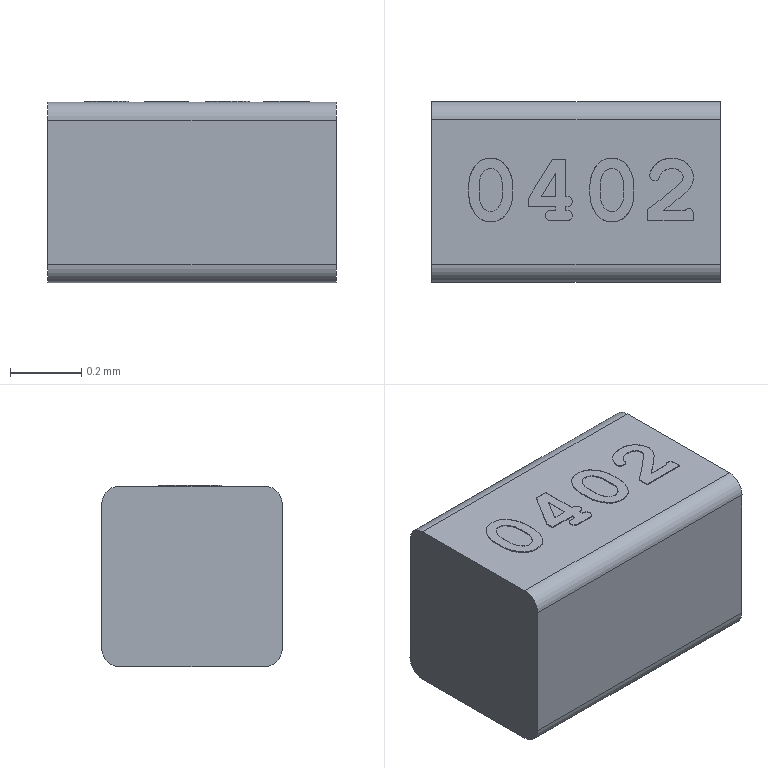Part | STEP file | RJ-USIO-V1_2-220411_24 | 3 solids | 92 faces | box 0.8128 x 0.508 x 0.5105 mm | volume 0.2081 mm3 | cylinder 45 | plane 39 | other 8 | commonest cylinder face diameters 0.03 x8 0.049 x6 0.05 x5 0.11 x5 0.102 x4 0.114 x4